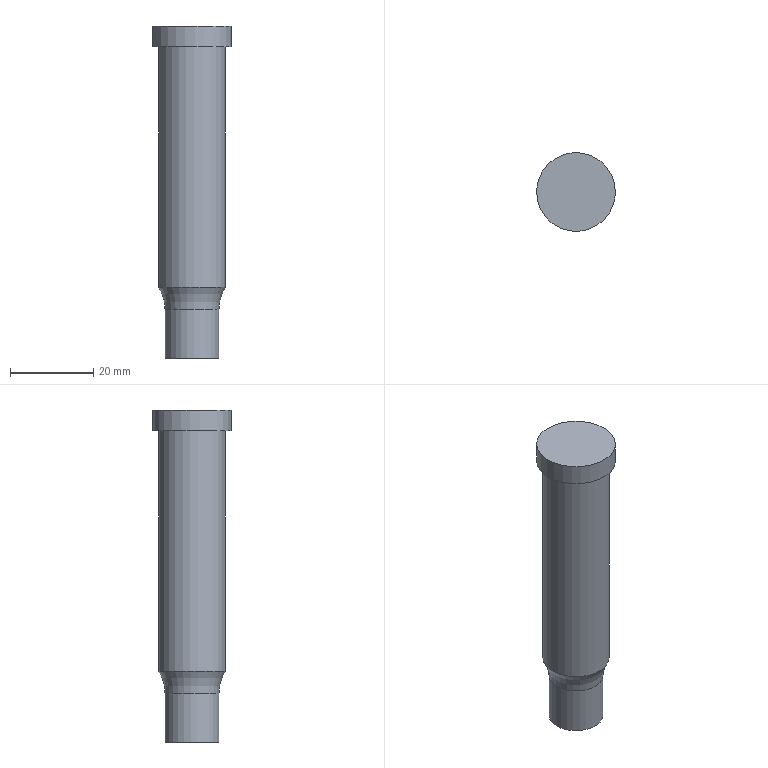Part | NX | features MAIN_BODY 2 | 1 solid | 7 faces | box 19 x 19 x 80 mm | volume 15447 mm3 | cylinder 3 | plane 3 | torus 1 | commonest cylinder face diameters 13 x1 16 x1 19 x1
STEP:
#1=CARTESIAN_POINT('',(1508.717,278.951,36.));
#2=VERTEX_POINT('',#1);
#3=CARTESIAN_POINT('',(1501.467,275.571,36.));
#4=DIRECTION('',(0.,0.,-1.));
#5=DIRECTION('',(0.9063,0.4226,0.));
#6=AXIS2_PLACEMENT_3D('',#3,#4,#5);
#7=CIRCLE('',#6,8.);
#8=EDGE_CURVE('',#2,#2,#7,.T.);
#9=ORIENTED_EDGE('',*,*,#8,.F.);
#10=EDGE_LOOP('',(#9));
#11=FACE_BOUND('',#10,.T.);
#12=CARTESIAN_POINT('',(1508.717,278.951,94.));
#13=VERTEX_POINT('',#12);
#14=CARTESIAN_POINT('',(1501.467,275.571,94.));
#15=DIRECTION('',(0.,0.,-1.));
#16=DIRECTION('',(0.9063,0.4226,0.));
#17=AXIS2_PLACEMENT_3D('',#14,#15,#16);
#18=CIRCLE('',#17,8.);
#19=EDGE_CURVE('',#13,#13,#18,.T.);
#20=ORIENTED_EDGE('',*,*,#19,.T.);
#21=EDGE_LOOP('',(#20));
#22=FACE_BOUND('',#21,.T.);
#23=CARTESIAN_POINT('',(1501.467,275.571,97.));
#24=DIRECTION('',(0.,0.,-1.));
#25=DIRECTION('',(-0.9063,-0.4226,0.));
#26=AXIS2_PLACEMENT_3D('',#23,#24,#25);
#27=CYLINDRICAL_SURFACE('',#26,8.);
#28=ADVANCED_FACE('',(#11,#22),#27,.T.);
#29=CARTESIAN_POINT('',(1510.076,279.585,94.));
#30=VERTEX_POINT('',#29);
#31=CARTESIAN_POINT('',(1501.467,275.571,94.));
#32=DIRECTION('',(0.,0.,-1.));
#33=DIRECTION('',(0.9063,0.4226,0.));
#34=AXIS2_PLACEMENT_3D('',#31,#32,#33);
#35=CIRCLE('',#34,9.5);
#36=EDGE_CURVE('',#30,#30,#35,.T.);
#37=ORIENTED_EDGE('',*,*,#36,.T.);
#38=EDGE_LOOP('',(#37));
#39=FACE_BOUND('',#38,.T.);
#40=ORIENTED_EDGE('',*,*,#19,.F.);
#41=EDGE_LOOP('',(#40));
#42=FACE_BOUND('',#41,.T.);
#43=CARTESIAN_POINT('',(1501.467,275.571,94.));
#44=DIRECTION('',(0.,0.,1.));
#45=DIRECTION('',(0.9063,0.4226,0.));
#46=AXIS2_PLACEMENT_3D('',#43,#44,#45);
#47=PLANE('',#46);
#48=ADVANCED_FACE('',(#39,#42),#47,.F.);
#49=ORIENTED_EDGE('',*,*,#36,.F.);
#50=EDGE_LOOP('',(#49));
#51=FACE_BOUND('',#50,.T.);
#52=CARTESIAN_POINT('',(1510.076,279.585,99.));
#53=VERTEX_POINT('',#52);
#54=CARTESIAN_POINT('',(1501.467,275.571,99.));
#55=DIRECTION('',(0.,0.,-1.));
#56=DIRECTION('',(0.9063,0.4226,0.));
#57=AXIS2_PLACEMENT_3D('',#54,#55,#56);
#58=CIRCLE('',#57,9.5);
#59=EDGE_CURVE('',#53,#53,#58,.T.);
#60=ORIENTED_EDGE('',*,*,#59,.T.);
#61=EDGE_LOOP('',(#60));
#62=FACE_BOUND('',#61,.T.);
#63=CARTESIAN_POINT('',(1501.467,275.571,94.));
#64=DIRECTION('',(0.,0.,1.));
#65=DIRECTION('',(0.9063,0.4226,0.));
#66=AXIS2_PLACEMENT_3D('',#63,#64,#65);
#67=CYLINDRICAL_SURFACE('',#66,9.5);
#68=ADVANCED_FACE('',(#51,#62),#67,.T.);
#69=ORIENTED_EDGE('',*,*,#59,.F.);
#70=EDGE_LOOP('',(#69));
#71=FACE_BOUND('',#70,.T.);
#72=CARTESIAN_POINT('',(1501.467,275.571,99.));
#73=DIRECTION('',(0.,0.,1.));
#74=DIRECTION('',(0.9063,0.4226,0.));
#75=AXIS2_PLACEMENT_3D('',#72,#73,#74);
#76=PLANE('',#75);
#77=ADVANCED_FACE('',(#71),#76,.T.);
#78=CARTESIAN_POINT('',(1507.358,278.318,30.732));
#79=VERTEX_POINT('',#78);
#80=CARTESIAN_POINT('',(1501.467,275.571,30.732));
#81=DIRECTION('',(0.,0.,-1.));
#82=DIRECTION('',(0.9063,0.4226,0.));
#83=AXIS2_PLACEMENT_3D('',#80,#81,#82);
#84=CIRCLE('',#83,6.5);
#85=EDGE_CURVE('',#79,#79,#84,.F.);
#86=ORIENTED_EDGE('',*,*,#85,.F.);
#87=EDGE_LOOP('',(#86));
#88=FACE_BOUND('',#87,.T.);
#89=CARTESIAN_POINT('',(1507.358,278.318,19.));
#90=VERTEX_POINT('',#89);
#91=CARTESIAN_POINT('',(1501.467,275.571,19.));
#92=DIRECTION('',(0.,0.,-1.));
#93=DIRECTION('',(0.9063,0.4226,0.));
#94=AXIS2_PLACEMENT_3D('',#91,#92,#93);
#95=CIRCLE('',#94,6.5);
#96=EDGE_CURVE('',#90,#90,#95,.T.);
#97=ORIENTED_EDGE('',*,*,#96,.F.);
#98=EDGE_LOOP('',(#97));
#99=FACE_BOUND('',#98,.T.);
#100=CARTESIAN_POINT('',(1501.467,275.571,17.));
#101=DIRECTION('',(0.,0.,1.));
#102=DIRECTION('',(0.9063,0.4226,0.));
#103=AXIS2_PLACEMENT_3D('',#100,#101,#102);
#104=CYLINDRICAL_SURFACE('',#103,6.5);
#105=ADVANCED_FACE('',(#88,#99),#104,.T.);
#106=ORIENTED_EDGE('',*,*,#96,.T.);
#107=EDGE_LOOP('',(#106));
#108=FACE_BOUND('',#107,.T.);
#109=CARTESIAN_POINT('',(1501.467,275.571,19.));
#110=DIRECTION('',(0.,0.,1.));
#111=DIRECTION('',(0.9063,0.4226,0.));
#112=AXIS2_PLACEMENT_3D('',#109,#110,#111);
#113=PLANE('',#112);
#114=ADVANCED_FACE('',(#108),#113,.F.);
#115=ORIENTED_EDGE('',*,*,#85,.T.);
#116=EDGE_LOOP('',(#115));
#117=FACE_BOUND('',#116,.T.);
#118=ORIENTED_EDGE('',*,*,#8,.T.);
#119=EDGE_LOOP('',(#118));
#120=FACE_BOUND('',#119,.T.);
#121=CARTESIAN_POINT('',(1501.467,275.571,30.732));
#122=DIRECTION('',(0.,0.,1.));
#123=DIRECTION('',(0.9063,0.4226,0.));
#124=AXIS2_PLACEMENT_3D('',#121,#122,#123);
#125=TOROIDAL_SURFACE('',#124,16.5,10.);
#126=ADVANCED_FACE('',(#117,#120),#125,.F.);
#127=CLOSED_SHELL('',(#28,#48,#68,#77,#105,#114,#126));
#128=MANIFOLD_SOLID_BREP('',#127);
#129=(LENGTH_UNIT()NAMED_UNIT(*)SI_UNIT(.MILLI.,.METRE.));
#130=UNCERTAINTY_MEASURE_WITH_UNIT(LENGTH_MEASURE(0.00001),#129,'','');
#131=(NAMED_UNIT(*)PLANE_ANGLE_UNIT()SI_UNIT($,.RADIAN.));
#132=(NAMED_UNIT(*)SI_UNIT($,.STERADIAN.)SOLID_ANGLE_UNIT());
#133=(GEOMETRIC_REPRESENTATION_CONTEXT(3)GLOBAL_UNCERTAINTY_ASSIGNED_CONTEXT((#130))GLOBAL_UNIT_ASSIGNED_CONTEXT((#129,#131,#132))REPRESENTATION_CONTEXT('',''));
#134=ADVANCED_BREP_SHAPE_REPRESENTATION('',(#128),#133);